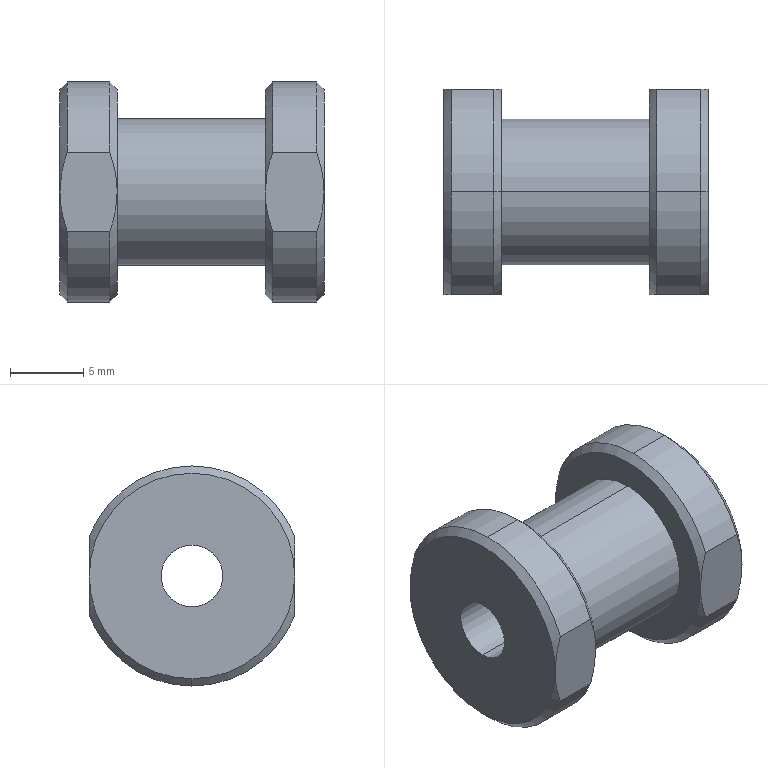Part | SolidWorks | features ICE 2, Chamfer 1, Extrusion 1, HoleWzd 1 | 1 solid | 30 faces | box 18 x 14 x 15 mm | volume 1893 mm3 | cone 12 | cylinder 10 | plane 8 | commonest cylinder face diameters 15 x6 4.2 x2 10 x2
STEP:
#1=CARTESIAN_POINT('',(3.9,0.,-5.));
#2=VERTEX_POINT('',#1);
#3=CARTESIAN_POINT('',(3.9,0.,5.));
#4=VERTEX_POINT('',#3);
#5=CARTESIAN_POINT('',(3.9,0.,0.));
#6=DIRECTION('',(1.,0.,0.));
#7=DIRECTION('',(0.,0.,-1.));
#8=AXIS2_PLACEMENT_3D('',#5,#6,#7);
#9=CIRCLE('',#8,5.);
#10=EDGE_CURVE('',#2,#4,#9,.T.);
#11=ORIENTED_EDGE('',*,*,#10,.T.);
#12=CARTESIAN_POINT('',(14.,0.,5.));
#13=VERTEX_POINT('',#12);
#14=CARTESIAN_POINT('',(3.9,0.,5.));
#15=DIRECTION('',(1.,0.,0.));
#16=VECTOR('',#15,1000.);
#17=LINE('',#14,#16);
#18=EDGE_CURVE('',#4,#13,#17,.T.);
#19=ORIENTED_EDGE('',*,*,#18,.T.);
#20=CARTESIAN_POINT('',(14.,0.,-5.));
#21=VERTEX_POINT('',#20);
#22=CARTESIAN_POINT('',(14.,0.,0.));
#23=DIRECTION('',(1.,0.,0.));
#24=DIRECTION('',(0.,0.,-1.));
#25=AXIS2_PLACEMENT_3D('',#22,#23,#24);
#26=CIRCLE('',#25,5.);
#27=EDGE_CURVE('',#21,#13,#26,.T.);
#28=ORIENTED_EDGE('',*,*,#27,.F.);
#29=CARTESIAN_POINT('',(3.9,0.,-5.));
#30=DIRECTION('',(1.,0.,0.));
#31=VECTOR('',#30,1000.);
#32=LINE('',#29,#31);
#33=EDGE_CURVE('',#2,#21,#32,.T.);
#34=ORIENTED_EDGE('',*,*,#33,.F.);
#35=EDGE_LOOP('',(#11,#19,#28,#34));
#36=FACE_OUTER_BOUND('',#35,.T.);
#37=CARTESIAN_POINT('',(3.9,0.,0.));
#38=DIRECTION('',(1.,0.,0.));
#39=DIRECTION('',(0.,0.,-1.));
#40=AXIS2_PLACEMENT_3D('',#37,#38,#39);
#41=CYLINDRICAL_SURFACE('',#40,5.);
#42=ADVANCED_FACE('',(#36),#41,.T.);
#43=CARTESIAN_POINT('',(0.,0.,2.1));
#44=VERTEX_POINT('',#43);
#45=CARTESIAN_POINT('',(0.,0.,-2.1));
#46=VERTEX_POINT('',#45);
#47=CARTESIAN_POINT('',(0.,0.,0.));
#48=DIRECTION('',(1.,0.,0.));
#49=DIRECTION('',(0.,0.,-1.));
#50=AXIS2_PLACEMENT_3D('',#47,#48,#49);
#51=CIRCLE('',#50,2.1);
#52=EDGE_CURVE('',#44,#46,#51,.T.);
#53=ORIENTED_EDGE('',*,*,#52,.F.);
#54=CARTESIAN_POINT('',(18.,0.,2.1));
#55=VERTEX_POINT('',#54);
#56=CARTESIAN_POINT('',(18.,0.,2.1));
#57=DIRECTION('',(1.,0.,0.));
#58=VECTOR('',#57,1000.);
#59=LINE('',#56,#58);
#60=EDGE_CURVE('',#44,#55,#59,.T.);
#61=ORIENTED_EDGE('',*,*,#60,.T.);
#62=CARTESIAN_POINT('',(18.,0.,-2.1));
#63=VERTEX_POINT('',#62);
#64=CARTESIAN_POINT('',(18.,0.,0.));
#65=DIRECTION('',(1.,0.,0.));
#66=DIRECTION('',(0.,0.,-1.));
#67=AXIS2_PLACEMENT_3D('',#64,#65,#66);
#68=CIRCLE('',#67,2.1);
#69=EDGE_CURVE('',#55,#63,#68,.T.);
#70=ORIENTED_EDGE('',*,*,#69,.T.);
#71=CARTESIAN_POINT('',(18.,0.,-2.1));
#72=DIRECTION('',(1.,0.,0.));
#73=VECTOR('',#72,1000.);
#74=LINE('',#71,#73);
#75=EDGE_CURVE('',#46,#63,#74,.T.);
#76=ORIENTED_EDGE('',*,*,#75,.F.);
#77=EDGE_LOOP('',(#53,#61,#70,#76));
#78=FACE_OUTER_BOUND('',#77,.T.);
#79=CARTESIAN_POINT('',(18.,0.,0.));
#80=DIRECTION('',(1.,0.,0.));
#81=DIRECTION('',(0.,0.,-1.));
#82=AXIS2_PLACEMENT_3D('',#79,#80,#81);
#83=CYLINDRICAL_SURFACE('',#82,2.1);
#84=ADVANCED_FACE('',(#78),#83,.F.);
#85=CARTESIAN_POINT('',(0.,0.,-7.));
#86=VERTEX_POINT('',#85);
#87=CARTESIAN_POINT('',(0.,-7.,0.));
#88=VERTEX_POINT('',#87);
#89=CARTESIAN_POINT('',(0.,0.,0.));
#90=DIRECTION('',(-1.,0.,0.));
#91=DIRECTION('',(0.,0.,-1.));
#92=AXIS2_PLACEMENT_3D('',#89,#90,#91);
#93=CIRCLE('',#92,7.);
#94=EDGE_CURVE('',#86,#88,#93,.T.);
#95=ORIENTED_EDGE('',*,*,#94,.F.);
#96=CARTESIAN_POINT('',(0.5,0.,-7.5));
#97=VERTEX_POINT('',#96);
#98=CARTESIAN_POINT('',(0.5,0.,-7.5));
#99=DIRECTION('',(0.7071,0.,-0.7071));
#100=VECTOR('',#99,1000.);
#101=LINE('',#98,#100);
#102=EDGE_CURVE('',#86,#97,#101,.T.);
#103=ORIENTED_EDGE('',*,*,#102,.T.);
#104=CARTESIAN_POINT('',(0.5,-7.,-2.693));
#105=VERTEX_POINT('',#104);
#106=CARTESIAN_POINT('',(0.5,0.,0.));
#107=DIRECTION('',(1.,0.,0.));
#108=DIRECTION('',(0.,0.,-1.));
#109=AXIS2_PLACEMENT_3D('',#106,#107,#108);
#110=CIRCLE('',#109,7.5);
#111=EDGE_CURVE('',#105,#97,#110,.T.);
#112=ORIENTED_EDGE('',*,*,#111,.F.);
#113=CARTESIAN_POINT('',(0.5,-7.,-2.693));
#114=CARTESIAN_POINT('',(0.3456,-7.,-2.263));
#115=CARTESIAN_POINT('',(0.2183,-7.,-1.816));
#116=CARTESIAN_POINT('',(0.04574,-7.,-0.9154));
#117=CARTESIAN_POINT('',(0.,-7.,-0.4603));
#118=CARTESIAN_POINT('',(0.,-7.,0.));
#119=B_SPLINE_CURVE_WITH_KNOTS('',3,(#113,#114,#115,#116,#117,#118),.UNSPECIFIED.,.F.,.F.,(4,2,4),(0.002778,0.004145,0.005512),.UNSPECIFIED.);
#120=EDGE_CURVE('',#105,#88,#119,.T.);
#121=ORIENTED_EDGE('',*,*,#120,.T.);
#122=EDGE_LOOP('',(#95,#103,#112,#121));
#123=FACE_OUTER_BOUND('',#122,.T.);
#124=CARTESIAN_POINT('',(0.5,0.,0.));
#125=DIRECTION('',(1.,0.,0.));
#126=DIRECTION('',(0.,0.,-1.));
#127=AXIS2_PLACEMENT_3D('',#124,#125,#126);
#128=CONICAL_SURFACE('',#127,7.5,0.7854);
#129=ADVANCED_FACE('',(#123),#128,.T.);
#130=CARTESIAN_POINT('',(3.9,0.,7.));
#131=VERTEX_POINT('',#130);
#132=CARTESIAN_POINT('',(3.9,-7.,0.));
#133=VERTEX_POINT('',#132);
#134=CARTESIAN_POINT('',(3.9,0.,0.));
#135=DIRECTION('',(1.,0.,0.));
#136=DIRECTION('',(0.,0.,-1.));
#137=AXIS2_PLACEMENT_3D('',#134,#135,#136);
#138=CIRCLE('',#137,7.);
#139=EDGE_CURVE('',#131,#133,#138,.T.);
#140=ORIENTED_EDGE('',*,*,#139,.F.);
#141=CARTESIAN_POINT('',(3.4,0.,7.5));
#142=VERTEX_POINT('',#141);
#143=CARTESIAN_POINT('',(3.9,0.,7.));
#144=DIRECTION('',(-0.7071,0.,0.7071));
#145=VECTOR('',#144,1000.);
#146=LINE('',#143,#145);
#147=EDGE_CURVE('',#131,#142,#146,.T.);
#148=ORIENTED_EDGE('',*,*,#147,.T.);
#149=CARTESIAN_POINT('',(3.4,-7.,2.693));
#150=VERTEX_POINT('',#149);
#151=CARTESIAN_POINT('',(3.4,0.,0.));
#152=DIRECTION('',(-1.,0.,0.));
#153=DIRECTION('',(0.,0.,-1.));
#154=AXIS2_PLACEMENT_3D('',#151,#152,#153);
#155=CIRCLE('',#154,7.5);
#156=EDGE_CURVE('',#150,#142,#155,.T.);
#157=ORIENTED_EDGE('',*,*,#156,.F.);
#158=CARTESIAN_POINT('',(3.4,-7.,2.693));
#159=CARTESIAN_POINT('',(3.556,-7.,2.258));
#160=CARTESIAN_POINT('',(3.681,-7.,1.818));
#161=CARTESIAN_POINT('',(3.81,-7.,1.145));
#162=CARTESIAN_POINT('',(3.844,-7.,0.919));
#163=CARTESIAN_POINT('',(3.888,-7.,0.4621));
#164=CARTESIAN_POINT('',(3.9,-7.,0.2303));
#165=CARTESIAN_POINT('',(3.9,-7.,0.));
#166=B_SPLINE_CURVE_WITH_KNOTS('',3,(#158,#159,#160,#161,#162,#163,#164,#165),.UNSPECIFIED.,.F.,.F.,(4,2,2,4),(0.006062,0.007422,0.008103,0.008783),.UNSPECIFIED.);
#167=EDGE_CURVE('',#150,#133,#166,.T.);
#168=ORIENTED_EDGE('',*,*,#167,.T.);
#169=EDGE_LOOP('',(#140,#148,#157,#168));
#170=FACE_OUTER_BOUND('',#169,.T.);
#171=CARTESIAN_POINT('',(3.9,0.,0.));
#172=DIRECTION('',(-1.,0.,0.));
#173=DIRECTION('',(0.,0.,1.));
#174=AXIS2_PLACEMENT_3D('',#171,#172,#173);
#175=CONICAL_SURFACE('',#174,7.,0.7854);
#176=ADVANCED_FACE('',(#170),#175,.T.);
#177=CARTESIAN_POINT('',(14.,0.,-7.));
#178=VERTEX_POINT('',#177);
#179=CARTESIAN_POINT('',(14.,-7.,0.));
#180=VERTEX_POINT('',#179);
#181=CARTESIAN_POINT('',(14.,0.,0.));
#182=DIRECTION('',(-1.,0.,0.));
#183=DIRECTION('',(0.,0.,-1.));
#184=AXIS2_PLACEMENT_3D('',#181,#182,#183);
#185=CIRCLE('',#184,7.);
#186=EDGE_CURVE('',#178,#180,#185,.T.);
#187=ORIENTED_EDGE('',*,*,#186,.F.);
#188=CARTESIAN_POINT('',(14.5,0.,-7.5));
#189=VERTEX_POINT('',#188);
#190=CARTESIAN_POINT('',(14.5,0.,-7.5));
#191=DIRECTION('',(0.7071,0.,-0.7071));
#192=VECTOR('',#191,1000.);
#193=LINE('',#190,#192);
#194=EDGE_CURVE('',#178,#189,#193,.T.);
#195=ORIENTED_EDGE('',*,*,#194,.T.);
#196=CARTESIAN_POINT('',(14.5,-7.,-2.693));
#197=VERTEX_POINT('',#196);
#198=CARTESIAN_POINT('',(14.5,0.,0.));
#199=DIRECTION('',(1.,0.,0.));
#200=DIRECTION('',(0.,0.,-1.));
#201=AXIS2_PLACEMENT_3D('',#198,#199,#200);
#202=CIRCLE('',#201,7.5);
#203=EDGE_CURVE('',#197,#189,#202,.T.);
#204=ORIENTED_EDGE('',*,*,#203,.F.);
#205=CARTESIAN_POINT('',(14.5,-7.,-2.693));
#206=CARTESIAN_POINT('',(14.346,-7.,-2.263));
#207=CARTESIAN_POINT('',(14.218,-7.,-1.816));
#208=CARTESIAN_POINT('',(14.046,-7.,-0.9154));
#209=CARTESIAN_POINT('',(14.,-7.,-0.4603));
#210=CARTESIAN_POINT('',(14.,-7.,0.));
#211=B_SPLINE_CURVE_WITH_KNOTS('',3,(#205,#206,#207,#208,#209,#210),.UNSPECIFIED.,.F.,.F.,(4,2,4),(0.002778,0.004145,0.005512),.UNSPECIFIED.);
#212=EDGE_CURVE('',#197,#180,#211,.T.);
#213=ORIENTED_EDGE('',*,*,#212,.T.);
#214=EDGE_LOOP('',(#187,#195,#204,#213));
#215=FACE_OUTER_BOUND('',#214,.T.);
#216=CARTESIAN_POINT('',(14.5,0.,0.));
#217=DIRECTION('',(1.,0.,0.));
#218=DIRECTION('',(0.,0.,-1.));
#219=AXIS2_PLACEMENT_3D('',#216,#217,#218);
#220=CONICAL_SURFACE('',#219,7.5,0.7854);
#221=ADVANCED_FACE('',(#215),#220,.T.);
#222=CARTESIAN_POINT('',(18.,0.,7.));
#223=VERTEX_POINT('',#222);
#224=CARTESIAN_POINT('',(18.,-7.,0.));
#225=VERTEX_POINT('',#224);
#226=CARTESIAN_POINT('',(18.,0.,0.));
#227=DIRECTION('',(1.,0.,0.));
#228=DIRECTION('',(0.,0.,-1.));
#229=AXIS2_PLACEMENT_3D('',#226,#227,#228);
#230=CIRCLE('',#229,7.);
#231=EDGE_CURVE('',#223,#225,#230,.T.);
#232=ORIENTED_EDGE('',*,*,#231,.F.);
#233=CARTESIAN_POINT('',(17.5,0.,7.5));
#234=VERTEX_POINT('',#233);
#235=CARTESIAN_POINT('',(18.,0.,7.));
#236=DIRECTION('',(-0.7071,0.,0.7071));
#237=VECTOR('',#236,1000.);
#238=LINE('',#235,#237);
#239=EDGE_CURVE('',#223,#234,#238,.T.);
#240=ORIENTED_EDGE('',*,*,#239,.T.);
#241=CARTESIAN_POINT('',(17.5,-7.,2.693));
#242=VERTEX_POINT('',#241);
#243=CARTESIAN_POINT('',(17.5,0.,0.));
#244=DIRECTION('',(-1.,0.,0.));
#245=DIRECTION('',(0.,0.,-1.));
#246=AXIS2_PLACEMENT_3D('',#243,#244,#245);
#247=CIRCLE('',#246,7.5);
#248=EDGE_CURVE('',#242,#234,#247,.T.);
#249=ORIENTED_EDGE('',*,*,#248,.F.);
#250=CARTESIAN_POINT('',(17.5,-7.,2.693));
#251=CARTESIAN_POINT('',(17.656,-7.,2.258));
#252=CARTESIAN_POINT('',(17.781,-7.,1.818));
#253=CARTESIAN_POINT('',(17.91,-7.,1.145));
#254=CARTESIAN_POINT('',(17.944,-7.,0.919));
#255=CARTESIAN_POINT('',(17.988,-7.,0.4621));
#256=CARTESIAN_POINT('',(18.,-7.,0.2303));
#257=CARTESIAN_POINT('',(18.,-7.,0.));
#258=B_SPLINE_CURVE_WITH_KNOTS('',3,(#250,#251,#252,#253,#254,#255,#256,#257),.UNSPECIFIED.,.F.,.F.,(4,2,2,4),(0.006062,0.007422,0.008103,0.008783),.UNSPECIFIED.);
#259=EDGE_CURVE('',#242,#225,#258,.T.);
#260=ORIENTED_EDGE('',*,*,#259,.T.);
#261=EDGE_LOOP('',(#232,#240,#249,#260));
#262=FACE_OUTER_BOUND('',#261,.T.);
#263=CARTESIAN_POINT('',(18.,0.,0.));
#264=DIRECTION('',(-1.,0.,0.));
#265=DIRECTION('',(0.,0.,1.));
#266=AXIS2_PLACEMENT_3D('',#263,#264,#265);
#267=CONICAL_SURFACE('',#266,7.,0.7854);
#268=ADVANCED_FACE('',(#262),#267,.T.);
#269=ORIENTED_EDGE('',*,*,#248,.T.);
#270=CARTESIAN_POINT('',(14.5,0.,7.5));
#271=VERTEX_POINT('',#270);
#272=CARTESIAN_POINT('',(18.,0.,7.5));
#273=DIRECTION('',(-1.,0.,0.));
#274=VECTOR('',#273,1000.);
#275=LINE('',#272,#274);
#276=EDGE_CURVE('',#234,#271,#275,.T.);
#277=ORIENTED_EDGE('',*,*,#276,.T.);
#278=CARTESIAN_POINT('',(14.5,-7.,2.693));
#279=VERTEX_POINT('',#278);
#280=CARTESIAN_POINT('',(14.5,0.,0.));
#281=DIRECTION('',(1.,0.,0.));
#282=DIRECTION('',(0.,0.,-1.));
#283=AXIS2_PLACEMENT_3D('',#280,#281,#282);
#284=CIRCLE('',#283,7.5);
#285=EDGE_CURVE('',#271,#279,#284,.T.);
#286=ORIENTED_EDGE('',*,*,#285,.T.);
#287=CARTESIAN_POINT('',(18.,-7.,2.693));
#288=DIRECTION('',(-1.,0.,0.));
#289=VECTOR('',#288,1000.);
#290=LINE('',#287,#289);
#291=EDGE_CURVE('',#242,#279,#290,.T.);
#292=ORIENTED_EDGE('',*,*,#291,.F.);
#293=EDGE_LOOP('',(#269,#277,#286,#292));
#294=FACE_OUTER_BOUND('',#293,.T.);
#295=CARTESIAN_POINT('',(18.,0.,0.));
#296=DIRECTION('',(-1.,0.,0.));
#297=DIRECTION('',(0.,0.,1.));
#298=AXIS2_PLACEMENT_3D('',#295,#296,#297);
#299=CYLINDRICAL_SURFACE('',#298,7.5);
#300=ADVANCED_FACE('',(#294),#299,.T.);
#301=ORIENTED_EDGE('',*,*,#156,.T.);
#302=CARTESIAN_POINT('',(0.5,0.,7.5));
#303=VERTEX_POINT('',#302);
#304=CARTESIAN_POINT('',(18.,0.,7.5));
#305=DIRECTION('',(-1.,0.,0.));
#306=VECTOR('',#305,1000.);
#307=LINE('',#304,#306);
#308=EDGE_CURVE('',#142,#303,#307,.T.);
#309=ORIENTED_EDGE('',*,*,#308,.T.);
#310=CARTESIAN_POINT('',(0.5,-7.,2.693));
#311=VERTEX_POINT('',#310);
#312=CARTESIAN_POINT('',(0.5,0.,0.));
#313=DIRECTION('',(1.,0.,0.));
#314=DIRECTION('',(0.,0.,-1.));
#315=AXIS2_PLACEMENT_3D('',#312,#313,#314);
#316=CIRCLE('',#315,7.5);
#317=EDGE_CURVE('',#303,#311,#316,.T.);
#318=ORIENTED_EDGE('',*,*,#317,.T.);
#319=CARTESIAN_POINT('',(18.,-7.,2.693));
#320=DIRECTION('',(-1.,0.,0.));
#321=VECTOR('',#320,1000.);
#322=LINE('',#319,#321);
#323=EDGE_CURVE('',#150,#311,#322,.T.);
#324=ORIENTED_EDGE('',*,*,#323,.F.);
#325=EDGE_LOOP('',(#301,#309,#318,#324));
#326=FACE_OUTER_BOUND('',#325,.T.);
#327=CARTESIAN_POINT('',(18.,0.,0.));
#328=DIRECTION('',(-1.,0.,0.));
#329=DIRECTION('',(0.,0.,1.));
#330=AXIS2_PLACEMENT_3D('',#327,#328,#329);
#331=CYLINDRICAL_SURFACE('',#330,7.5);
#332=ADVANCED_FACE('',(#326),#331,.T.);
#333=ORIENTED_EDGE('',*,*,#308,.F.);
#334=CARTESIAN_POINT('',(3.4,7.,2.693));
#335=VERTEX_POINT('',#334);
#336=CARTESIAN_POINT('',(3.4,0.,0.));
#337=DIRECTION('',(-1.,0.,0.));
#338=DIRECTION('',(0.,0.,-1.));
#339=AXIS2_PLACEMENT_3D('',#336,#337,#338);
#340=CIRCLE('',#339,7.5);
#341=EDGE_CURVE('',#142,#335,#340,.T.);
#342=ORIENTED_EDGE('',*,*,#341,.T.);
#343=CARTESIAN_POINT('',(0.5,7.,2.693));
#344=VERTEX_POINT('',#343);
#345=CARTESIAN_POINT('',(18.,7.,2.693));
#346=DIRECTION('',(1.,0.,0.));
#347=VECTOR('',#346,1000.);
#348=LINE('',#345,#347);
#349=EDGE_CURVE('',#344,#335,#348,.T.);
#350=ORIENTED_EDGE('',*,*,#349,.F.);
#351=CARTESIAN_POINT('',(0.5,0.,0.));
#352=DIRECTION('',(1.,0.,0.));
#353=DIRECTION('',(0.,0.,-1.));
#354=AXIS2_PLACEMENT_3D('',#351,#352,#353);
#355=CIRCLE('',#354,7.5);
#356=EDGE_CURVE('',#344,#303,#355,.T.);
#357=ORIENTED_EDGE('',*,*,#356,.T.);
#358=EDGE_LOOP('',(#333,#342,#350,#357));
#359=FACE_OUTER_BOUND('',#358,.T.);
#360=CARTESIAN_POINT('',(18.,0.,0.));
#361=DIRECTION('',(-1.,0.,0.));
#362=DIRECTION('',(0.,0.,1.));
#363=AXIS2_PLACEMENT_3D('',#360,#361,#362);
#364=CYLINDRICAL_SURFACE('',#363,7.5);
#365=ADVANCED_FACE('',(#359),#364,.T.);
#366=CARTESIAN_POINT('',(3.4,-7.,-2.693));
#367=VERTEX_POINT('',#366);
#368=CARTESIAN_POINT('',(18.,-7.,-2.693));
#369=DIRECTION('',(1.,0.,0.));
#370=VECTOR('',#369,1000.);
#371=LINE('',#368,#370);
#372=EDGE_CURVE('',#105,#367,#371,.T.);
#373=ORIENTED_EDGE('',*,*,#372,.F.);
#374=ORIENTED_EDGE('',*,*,#111,.T.);
#375=CARTESIAN_POINT('',(0.5,7.,-2.693));
#376=VERTEX_POINT('',#375);
#377=CARTESIAN_POINT('',(0.5,0.,0.));
#378=DIRECTION('',(1.,0.,0.));
#379=DIRECTION('',(0.,0.,-1.));
#380=AXIS2_PLACEMENT_3D('',#377,#378,#379);
#381=CIRCLE('',#380,7.5);
#382=EDGE_CURVE('',#97,#376,#381,.T.);
#383=ORIENTED_EDGE('',*,*,#382,.T.);
#384=CARTESIAN_POINT('',(3.4,7.,-2.693));
#385=VERTEX_POINT('',#384);
#386=CARTESIAN_POINT('',(18.,7.,-2.693));
#387=DIRECTION('',(-1.,0.,0.));
#388=VECTOR('',#387,1000.);
#389=LINE('',#386,#388);
#390=EDGE_CURVE('',#385,#376,#389,.T.);
#391=ORIENTED_EDGE('',*,*,#390,.F.);
#392=CARTESIAN_POINT('',(3.4,0.,0.));
#393=DIRECTION('',(-1.,0.,0.));
#394=DIRECTION('',(0.,0.,-1.));
#395=AXIS2_PLACEMENT_3D('',#392,#393,#394);
#396=CIRCLE('',#395,7.5);
#397=EDGE_CURVE('',#385,#367,#396,.T.);
#398=ORIENTED_EDGE('',*,*,#397,.T.);
#399=EDGE_LOOP('',(#373,#374,#383,#391,#398));
#400=FACE_OUTER_BOUND('',#399,.T.);
#401=CARTESIAN_POINT('',(18.,0.,0.));
#402=DIRECTION('',(-1.,0.,0.));
#403=DIRECTION('',(0.,0.,1.));
#404=AXIS2_PLACEMENT_3D('',#401,#402,#403);
#405=CYLINDRICAL_SURFACE('',#404,7.5);
#406=ADVANCED_FACE('',(#400),#405,.T.);
#407=ORIENTED_EDGE('',*,*,#276,.F.);
#408=CARTESIAN_POINT('',(17.5,7.,2.693));
#409=VERTEX_POINT('',#408);
#410=CARTESIAN_POINT('',(17.5,0.,0.));
#411=DIRECTION('',(-1.,0.,0.));
#412=DIRECTION('',(0.,0.,-1.));
#413=AXIS2_PLACEMENT_3D('',#410,#411,#412);
#414=CIRCLE('',#413,7.5);
#415=EDGE_CURVE('',#234,#409,#414,.T.);
#416=ORIENTED_EDGE('',*,*,#415,.T.);
#417=CARTESIAN_POINT('',(14.5,7.,2.693));
#418=VERTEX_POINT('',#417);
#419=CARTESIAN_POINT('',(18.,7.,2.693));
#420=DIRECTION('',(1.,0.,0.));
#421=VECTOR('',#420,1000.);
#422=LINE('',#419,#421);
#423=EDGE_CURVE('',#418,#409,#422,.T.);
#424=ORIENTED_EDGE('',*,*,#423,.F.);
#425=CARTESIAN_POINT('',(14.5,0.,0.));
#426=DIRECTION('',(1.,0.,0.));
#427=DIRECTION('',(0.,0.,-1.));
#428=AXIS2_PLACEMENT_3D('',#425,#426,#427);
#429=CIRCLE('',#428,7.5);
#430=EDGE_CURVE('',#418,#271,#429,.T.);
#431=ORIENTED_EDGE('',*,*,#430,.T.);
#432=EDGE_LOOP('',(#407,#416,#424,#431));
#433=FACE_OUTER_BOUND('',#432,.T.);
#434=CARTESIAN_POINT('',(18.,0.,0.));
#435=DIRECTION('',(-1.,0.,0.));
#436=DIRECTION('',(0.,0.,1.));
#437=AXIS2_PLACEMENT_3D('',#434,#435,#436);
#438=CYLINDRICAL_SURFACE('',#437,7.5);
#439=ADVANCED_FACE('',(#433),#438,.T.);
#440=CARTESIAN_POINT('',(17.5,-7.,-2.693));
#441=VERTEX_POINT('',#440);
#442=CARTESIAN_POINT('',(18.,-7.,-2.693));
#443=DIRECTION('',(1.,0.,0.));
#444=VECTOR('',#443,1000.);
#445=LINE('',#442,#444);
#446=EDGE_CURVE('',#197,#441,#445,.T.);
#447=ORIENTED_EDGE('',*,*,#446,.F.);
#448=ORIENTED_EDGE('',*,*,#203,.T.);
#449=CARTESIAN_POINT('',(14.5,7.,-2.693));
#450=VERTEX_POINT('',#449);
#451=CARTESIAN_POINT('',(14.5,0.,0.));
#452=DIRECTION('',(1.,0.,0.));
#453=DIRECTION('',(0.,0.,-1.));
#454=AXIS2_PLACEMENT_3D('',#451,#452,#453);
#455=CIRCLE('',#454,7.5);
#456=EDGE_CURVE('',#189,#450,#455,.T.);
#457=ORIENTED_EDGE('',*,*,#456,.T.);
#458=CARTESIAN_POINT('',(17.5,7.,-2.693));
#459=VERTEX_POINT('',#458);
#460=CARTESIAN_POINT('',(18.,7.,-2.693));
#461=DIRECTION('',(-1.,0.,0.));
#462=VECTOR('',#461,1000.);
#463=LINE('',#460,#462);
#464=EDGE_CURVE('',#459,#450,#463,.T.);
#465=ORIENTED_EDGE('',*,*,#464,.F.);
#466=CARTESIAN_POINT('',(17.5,0.,0.));
#467=DIRECTION('',(-1.,0.,0.));
#468=DIRECTION('',(0.,0.,-1.));
#469=AXIS2_PLACEMENT_3D('',#466,#467,#468);
#470=CIRCLE('',#469,7.5);
#471=EDGE_CURVE('',#459,#441,#470,.T.);
#472=ORIENTED_EDGE('',*,*,#471,.T.);
#473=EDGE_LOOP('',(#447,#448,#457,#465,#472));
#474=FACE_OUTER_BOUND('',#473,.T.);
#475=CARTESIAN_POINT('',(18.,0.,0.));
#476=DIRECTION('',(-1.,0.,0.));
#477=DIRECTION('',(0.,0.,1.));
#478=AXIS2_PLACEMENT_3D('',#475,#476,#477);
#479=CYLINDRICAL_SURFACE('',#478,7.5);
#480=ADVANCED_FACE('',(#474),#479,.T.);
#481=ORIENTED_EDGE('',*,*,#239,.F.);
#482=CARTESIAN_POINT('',(18.,7.,0.));
#483=VERTEX_POINT('',#482);
#484=CARTESIAN_POINT('',(18.,0.,0.));
#485=DIRECTION('',(1.,0.,0.));
#486=DIRECTION('',(0.,0.,-1.));
#487=AXIS2_PLACEMENT_3D('',#484,#485,#486);
#488=CIRCLE('',#487,7.);
#489=EDGE_CURVE('',#483,#223,#488,.T.);
#490=ORIENTED_EDGE('',*,*,#489,.F.);
#491=CARTESIAN_POINT('',(18.,7.,0.));
#492=CARTESIAN_POINT('',(18.,7.,0.2303));
#493=CARTESIAN_POINT('',(17.988,7.,0.4621));
#494=CARTESIAN_POINT('',(17.944,7.,0.919));
#495=CARTESIAN_POINT('',(17.91,7.,1.145));
#496=CARTESIAN_POINT('',(17.781,7.,1.818));
#497=CARTESIAN_POINT('',(17.656,7.,2.258));
#498=CARTESIAN_POINT('',(17.5,7.,2.693));
#499=B_SPLINE_CURVE_WITH_KNOTS('',3,(#491,#492,#493,#494,#495,#496,#497,#498),.UNSPECIFIED.,.F.,.F.,(4,2,2,4),(0.005512,0.006196,0.00688,0.008248),.UNSPECIFIED.);
#500=EDGE_CURVE('',#483,#409,#499,.T.);
#501=ORIENTED_EDGE('',*,*,#500,.T.);
#502=ORIENTED_EDGE('',*,*,#415,.F.);
#503=EDGE_LOOP('',(#481,#490,#501,#502));
#504=FACE_OUTER_BOUND('',#503,.T.);
#505=CARTESIAN_POINT('',(18.,0.,0.));
#506=DIRECTION('',(-1.,0.,0.));
#507=DIRECTION('',(0.,0.,1.));
#508=AXIS2_PLACEMENT_3D('',#505,#506,#507);
#509=CONICAL_SURFACE('',#508,7.,0.7854);
#510=ADVANCED_FACE('',(#504),#509,.T.);
#511=CARTESIAN_POINT('',(18.,0.,0.));
#512=DIRECTION('',(1.,0.,0.));
#513=DIRECTION('',(0.,0.,-1.));
#514=AXIS2_PLACEMENT_3D('',#511,#512,#513);
#515=CIRCLE('',#514,7.);
#516=EDGE_CURVE('',#225,#483,#515,.T.);
#517=ORIENTED_EDGE('',*,*,#516,.F.);
#518=CARTESIAN_POINT('',(18.,-7.,0.));
#519=CARTESIAN_POINT('',(18.,-7.,-0.4603));
#520=CARTESIAN_POINT('',(17.954,-7.,-0.9154));
#521=CARTESIAN_POINT('',(17.782,-7.,-1.816));
#522=CARTESIAN_POINT('',(17.654,-7.,-2.263));
#523=CARTESIAN_POINT('',(17.5,-7.,-2.693));
#524=B_SPLINE_CURVE_WITH_KNOTS('',3,(#518,#519,#520,#521,#522,#523),.UNSPECIFIED.,.F.,.F.,(4,2,4),(0.008783,0.01014,0.0115),.UNSPECIFIED.);
#525=EDGE_CURVE('',#225,#441,#524,.T.);
#526=ORIENTED_EDGE('',*,*,#525,.T.);
#527=ORIENTED_EDGE('',*,*,#471,.F.);
#528=CARTESIAN_POINT('',(17.5,7.,-2.693));
#529=CARTESIAN_POINT('',(17.654,7.,-2.263));
#530=CARTESIAN_POINT('',(17.782,7.,-1.816));
#531=CARTESIAN_POINT('',(17.954,7.,-0.9154));
#532=CARTESIAN_POINT('',(18.,7.,-0.4603));
#533=CARTESIAN_POINT('',(18.,7.,0.));
#534=B_SPLINE_CURVE_WITH_KNOTS('',3,(#528,#529,#530,#531,#532,#533),.UNSPECIFIED.,.F.,.F.,(4,2,4),(0.002778,0.004145,0.005512),.UNSPECIFIED.);
#535=EDGE_CURVE('',#459,#483,#534,.T.);
#536=ORIENTED_EDGE('',*,*,#535,.T.);
#537=EDGE_LOOP('',(#517,#526,#527,#536));
#538=FACE_OUTER_BOUND('',#537,.T.);
#539=CARTESIAN_POINT('',(18.,0.,0.));
#540=DIRECTION('',(-1.,0.,0.));
#541=DIRECTION('',(0.,0.,1.));
#542=AXIS2_PLACEMENT_3D('',#539,#540,#541);
#543=CONICAL_SURFACE('',#542,7.,0.7854);
#544=ADVANCED_FACE('',(#538),#543,.T.);
#545=ORIENTED_EDGE('',*,*,#194,.F.);
#546=CARTESIAN_POINT('',(14.,7.,0.));
#547=VERTEX_POINT('',#546);
#548=CARTESIAN_POINT('',(14.,0.,0.));
#549=DIRECTION('',(-1.,0.,0.));
#550=DIRECTION('',(0.,0.,-1.));
#551=AXIS2_PLACEMENT_3D('',#548,#549,#550);
#552=CIRCLE('',#551,7.);
#553=EDGE_CURVE('',#547,#178,#552,.T.);
#554=ORIENTED_EDGE('',*,*,#553,.F.);
#555=CARTESIAN_POINT('',(14.,7.,0.));
#556=CARTESIAN_POINT('',(14.,7.,-0.4603));
#557=CARTESIAN_POINT('',(14.046,7.,-0.9154));
#558=CARTESIAN_POINT('',(14.218,7.,-1.816));
#559=CARTESIAN_POINT('',(14.346,7.,-2.263));
#560=CARTESIAN_POINT('',(14.5,7.,-2.693));
#561=B_SPLINE_CURVE_WITH_KNOTS('',3,(#555,#556,#557,#558,#559,#560),.UNSPECIFIED.,.F.,.F.,(4,2,4),(0.008783,0.01014,0.0115),.UNSPECIFIED.);
#562=EDGE_CURVE('',#547,#450,#561,.T.);
#563=ORIENTED_EDGE('',*,*,#562,.T.);
#564=ORIENTED_EDGE('',*,*,#456,.F.);
#565=EDGE_LOOP('',(#545,#554,#563,#564));
#566=FACE_OUTER_BOUND('',#565,.T.);
#567=CARTESIAN_POINT('',(14.5,0.,0.));
#568=DIRECTION('',(1.,0.,0.));
#569=DIRECTION('',(0.,0.,-1.));
#570=AXIS2_PLACEMENT_3D('',#567,#568,#569);
#571=CONICAL_SURFACE('',#570,7.5,0.7854);
#572=ADVANCED_FACE('',(#566),#571,.T.);
#573=CARTESIAN_POINT('',(14.,0.,0.));
#574=DIRECTION('',(-1.,0.,0.));
#575=DIRECTION('',(0.,0.,-1.));
#576=AXIS2_PLACEMENT_3D('',#573,#574,#575);
#577=CIRCLE('',#576,7.);
#578=EDGE_CURVE('',#180,#547,#577,.T.);
#579=ORIENTED_EDGE('',*,*,#578,.F.);
#580=CARTESIAN_POINT('',(14.,-7.,0.));
#581=CARTESIAN_POINT('',(14.,-7.,0.2303));
#582=CARTESIAN_POINT('',(14.012,-7.,0.4621));
#583=CARTESIAN_POINT('',(14.056,-7.,0.919));
#584=CARTESIAN_POINT('',(14.09,-7.,1.145));
#585=CARTESIAN_POINT('',(14.219,-7.,1.818));
#586=CARTESIAN_POINT('',(14.344,-7.,2.258));
#587=CARTESIAN_POINT('',(14.5,-7.,2.693));
#588=B_SPLINE_CURVE_WITH_KNOTS('',3,(#580,#581,#582,#583,#584,#585,#586,#587),.UNSPECIFIED.,.F.,.F.,(4,2,2,4),(0.005512,0.006196,0.00688,0.008248),.UNSPECIFIED.);
#589=EDGE_CURVE('',#180,#279,#588,.T.);
#590=ORIENTED_EDGE('',*,*,#589,.T.);
#591=ORIENTED_EDGE('',*,*,#285,.F.);
#592=ORIENTED_EDGE('',*,*,#430,.F.);
#593=CARTESIAN_POINT('',(14.5,7.,2.693));
#594=CARTESIAN_POINT('',(14.344,7.,2.258));
#595=CARTESIAN_POINT('',(14.219,7.,1.818));
#596=CARTESIAN_POINT('',(14.09,7.,1.145));
#597=CARTESIAN_POINT('',(14.056,7.,0.919));
#598=CARTESIAN_POINT('',(14.012,7.,0.4621));
#599=CARTESIAN_POINT('',(14.,7.,0.2303));
#600=CARTESIAN_POINT('',(14.,7.,0.));
#601=B_SPLINE_CURVE_WITH_KNOTS('',3,(#593,#594,#595,#596,#597,#598,#599,#600),.UNSPECIFIED.,.F.,.F.,(4,2,2,4),(0.006062,0.007422,0.008103,0.008783),.UNSPECIFIED.);
#602=EDGE_CURVE('',#418,#547,#601,.T.);
#603=ORIENTED_EDGE('',*,*,#602,.T.);
#604=EDGE_LOOP('',(#579,#590,#591,#592,#603));
#605=FACE_OUTER_BOUND('',#604,.T.);
#606=CARTESIAN_POINT('',(14.5,0.,0.));
#607=DIRECTION('',(1.,0.,0.));
#608=DIRECTION('',(0.,0.,-1.));
#609=AXIS2_PLACEMENT_3D('',#606,#607,#608);
#610=CONICAL_SURFACE('',#609,7.5,0.7854);
#611=ADVANCED_FACE('',(#605),#610,.T.);
#612=ORIENTED_EDGE('',*,*,#147,.F.);
#613=CARTESIAN_POINT('',(3.9,7.,0.));
#614=VERTEX_POINT('',#613);
#615=CARTESIAN_POINT('',(3.9,0.,0.));
#616=DIRECTION('',(1.,0.,0.));
#617=DIRECTION('',(0.,0.,-1.));
#618=AXIS2_PLACEMENT_3D('',#615,#616,#617);
#619=CIRCLE('',#618,7.);
#620=EDGE_CURVE('',#614,#131,#619,.T.);
#621=ORIENTED_EDGE('',*,*,#620,.F.);
#622=CARTESIAN_POINT('',(3.9,7.,0.));
#623=CARTESIAN_POINT('',(3.9,7.,0.2303));
#624=CARTESIAN_POINT('',(3.888,7.,0.4621));
#625=CARTESIAN_POINT('',(3.844,7.,0.919));
#626=CARTESIAN_POINT('',(3.81,7.,1.145));
#627=CARTESIAN_POINT('',(3.681,7.,1.818));
#628=CARTESIAN_POINT('',(3.556,7.,2.258));
#629=CARTESIAN_POINT('',(3.4,7.,2.693));
#630=B_SPLINE_CURVE_WITH_KNOTS('',3,(#622,#623,#624,#625,#626,#627,#628,#629),.UNSPECIFIED.,.F.,.F.,(4,2,2,4),(0.005512,0.006196,0.00688,0.008248),.UNSPECIFIED.);
#631=EDGE_CURVE('',#614,#335,#630,.T.);
#632=ORIENTED_EDGE('',*,*,#631,.T.);
#633=ORIENTED_EDGE('',*,*,#341,.F.);
#634=EDGE_LOOP('',(#612,#621,#632,#633));
#635=FACE_OUTER_BOUND('',#634,.T.);
#636=CARTESIAN_POINT('',(3.9,0.,0.));
#637=DIRECTION('',(-1.,0.,0.));
#638=DIRECTION('',(0.,0.,1.));
#639=AXIS2_PLACEMENT_3D('',#636,#637,#638);
#640=CONICAL_SURFACE('',#639,7.,0.7854);
#641=ADVANCED_FACE('',(#635),#640,.T.);
#642=CARTESIAN_POINT('',(3.9,0.,0.));
#643=DIRECTION('',(1.,0.,0.));
#644=DIRECTION('',(0.,0.,-1.));
#645=AXIS2_PLACEMENT_3D('',#642,#643,#644);
#646=CIRCLE('',#645,7.);
#647=EDGE_CURVE('',#133,#614,#646,.T.);
#648=ORIENTED_EDGE('',*,*,#647,.F.);
#649=CARTESIAN_POINT('',(3.9,-7.,0.));
#650=CARTESIAN_POINT('',(3.9,-7.,-0.4603));
#651=CARTESIAN_POINT('',(3.854,-7.,-0.9154));
#652=CARTESIAN_POINT('',(3.682,-7.,-1.816));
#653=CARTESIAN_POINT('',(3.554,-7.,-2.263));
#654=CARTESIAN_POINT('',(3.4,-7.,-2.693));
#655=B_SPLINE_CURVE_WITH_KNOTS('',3,(#649,#650,#651,#652,#653,#654),.UNSPECIFIED.,.F.,.F.,(4,2,4),(0.008783,0.01014,0.0115),.UNSPECIFIED.);
#656=EDGE_CURVE('',#133,#367,#655,.T.);
#657=ORIENTED_EDGE('',*,*,#656,.T.);
#658=ORIENTED_EDGE('',*,*,#397,.F.);
#659=CARTESIAN_POINT('',(3.4,7.,-2.693));
#660=CARTESIAN_POINT('',(3.554,7.,-2.263));
#661=CARTESIAN_POINT('',(3.682,7.,-1.816));
#662=CARTESIAN_POINT('',(3.854,7.,-0.9154));
#663=CARTESIAN_POINT('',(3.9,7.,-0.4603));
#664=CARTESIAN_POINT('',(3.9,7.,0.));
#665=B_SPLINE_CURVE_WITH_KNOTS('',3,(#659,#660,#661,#662,#663,#664),.UNSPECIFIED.,.F.,.F.,(4,2,4),(0.002778,0.004145,0.005512),.UNSPECIFIED.);
#666=EDGE_CURVE('',#385,#614,#665,.T.);
#667=ORIENTED_EDGE('',*,*,#666,.T.);
#668=EDGE_LOOP('',(#648,#657,#658,#667));
#669=FACE_OUTER_BOUND('',#668,.T.);
#670=CARTESIAN_POINT('',(3.9,0.,0.));
#671=DIRECTION('',(-1.,0.,0.));
#672=DIRECTION('',(0.,0.,1.));
#673=AXIS2_PLACEMENT_3D('',#670,#671,#672);
#674=CONICAL_SURFACE('',#673,7.,0.7854);
#675=ADVANCED_FACE('',(#669),#674,.T.);
#676=ORIENTED_EDGE('',*,*,#102,.F.);
#677=CARTESIAN_POINT('',(0.,7.,0.));
#678=VERTEX_POINT('',#677);
#679=CARTESIAN_POINT('',(0.,0.,0.));
#680=DIRECTION('',(-1.,0.,0.));
#681=DIRECTION('',(0.,0.,-1.));
#682=AXIS2_PLACEMENT_3D('',#679,#680,#681);
#683=CIRCLE('',#682,7.);
#684=EDGE_CURVE('',#678,#86,#683,.T.);
#685=ORIENTED_EDGE('',*,*,#684,.F.);
#686=CARTESIAN_POINT('',(0.,7.,0.));
#687=CARTESIAN_POINT('',(0.,7.,-0.4603));
#688=CARTESIAN_POINT('',(0.04574,7.,-0.9154));
#689=CARTESIAN_POINT('',(0.2183,7.,-1.816));
#690=CARTESIAN_POINT('',(0.3456,7.,-2.263));
#691=CARTESIAN_POINT('',(0.5,7.,-2.693));
#692=B_SPLINE_CURVE_WITH_KNOTS('',3,(#686,#687,#688,#689,#690,#691),.UNSPECIFIED.,.F.,.F.,(4,2,4),(0.008783,0.01014,0.0115),.UNSPECIFIED.);
#693=EDGE_CURVE('',#678,#376,#692,.T.);
#694=ORIENTED_EDGE('',*,*,#693,.T.);
#695=ORIENTED_EDGE('',*,*,#382,.F.);
#696=EDGE_LOOP('',(#676,#685,#694,#695));
#697=FACE_OUTER_BOUND('',#696,.T.);
#698=CARTESIAN_POINT('',(0.5,0.,0.));
#699=DIRECTION('',(1.,0.,0.));
#700=DIRECTION('',(0.,0.,-1.));
#701=AXIS2_PLACEMENT_3D('',#698,#699,#700);
#702=CONICAL_SURFACE('',#701,7.5,0.7854);
#703=ADVANCED_FACE('',(#697),#702,.T.);
#704=CARTESIAN_POINT('',(0.,0.,0.));
#705=DIRECTION('',(-1.,0.,0.));
#706=DIRECTION('',(0.,0.,-1.));
#707=AXIS2_PLACEMENT_3D('',#704,#705,#706);
#708=CIRCLE('',#707,7.);
#709=EDGE_CURVE('',#88,#678,#708,.T.);
#710=ORIENTED_EDGE('',*,*,#709,.F.);
#711=CARTESIAN_POINT('',(0.,-7.,0.));
#712=CARTESIAN_POINT('',(0.,-7.,0.2303));
#713=CARTESIAN_POINT('',(0.01156,-7.,0.4621));
#714=CARTESIAN_POINT('',(0.05641,-7.,0.919));
#715=CARTESIAN_POINT('',(0.08965,-7.,1.145));
#716=CARTESIAN_POINT('',(0.2188,-7.,1.818));
#717=CARTESIAN_POINT('',(0.3441,-7.,2.258));
#718=CARTESIAN_POINT('',(0.5,-7.,2.693));
#719=B_SPLINE_CURVE_WITH_KNOTS('',3,(#711,#712,#713,#714,#715,#716,#717,#718),.UNSPECIFIED.,.F.,.F.,(4,2,2,4),(0.005512,0.006196,0.00688,0.008248),.UNSPECIFIED.);
#720=EDGE_CURVE('',#88,#311,#719,.T.);
#721=ORIENTED_EDGE('',*,*,#720,.T.);
#722=ORIENTED_EDGE('',*,*,#317,.F.);
#723=ORIENTED_EDGE('',*,*,#356,.F.);
#724=CARTESIAN_POINT('',(0.5,7.,2.693));
#725=CARTESIAN_POINT('',(0.3441,7.,2.258));
#726=CARTESIAN_POINT('',(0.2188,7.,1.818));
#727=CARTESIAN_POINT('',(0.08965,7.,1.145));
#728=CARTESIAN_POINT('',(0.05641,7.,0.919));
#729=CARTESIAN_POINT('',(0.01156,7.,0.4621));
#730=CARTESIAN_POINT('',(0.,7.,0.2303));
#731=CARTESIAN_POINT('',(0.,7.,0.));
#732=B_SPLINE_CURVE_WITH_KNOTS('',3,(#724,#725,#726,#727,#728,#729,#730,#731),.UNSPECIFIED.,.F.,.F.,(4,2,2,4),(0.006062,0.007422,0.008103,0.008783),.UNSPECIFIED.);
#733=EDGE_CURVE('',#344,#678,#732,.T.);
#734=ORIENTED_EDGE('',*,*,#733,.T.);
#735=EDGE_LOOP('',(#710,#721,#722,#723,#734));
#736=FACE_OUTER_BOUND('',#735,.T.);
#737=CARTESIAN_POINT('',(0.5,0.,0.));
#738=DIRECTION('',(1.,0.,0.));
#739=DIRECTION('',(0.,0.,-1.));
#740=AXIS2_PLACEMENT_3D('',#737,#738,#739);
#741=CONICAL_SURFACE('',#740,7.5,0.7854);
#742=ADVANCED_FACE('',(#736),#741,.T.);
#743=ORIENTED_EDGE('',*,*,#489,.T.);
#744=ORIENTED_EDGE('',*,*,#231,.T.);
#745=ORIENTED_EDGE('',*,*,#516,.T.);
#746=EDGE_LOOP('',(#743,#744,#745));
#747=FACE_OUTER_BOUND('',#746,.T.);
#748=CARTESIAN_POINT('',(18.,0.,0.));
#749=DIRECTION('',(1.,0.,0.));
#750=DIRECTION('',(0.,0.,-1.));
#751=AXIS2_PLACEMENT_3D('',#748,#749,#750);
#752=CIRCLE('',#751,2.1);
#753=EDGE_CURVE('',#63,#55,#752,.T.);
#754=ORIENTED_EDGE('',*,*,#753,.F.);
#755=ORIENTED_EDGE('',*,*,#69,.F.);
#756=EDGE_LOOP('',(#754,#755));
#757=FACE_BOUND('',#756,.T.);
#758=CARTESIAN_POINT('',(18.,0.,0.));
#759=DIRECTION('',(1.,0.,0.));
#760=DIRECTION('',(0.,0.,-1.));
#761=AXIS2_PLACEMENT_3D('',#758,#759,#760);
#762=PLANE('',#761);
#763=ADVANCED_FACE('',(#747,#757),#762,.T.);
#764=ORIENTED_EDGE('',*,*,#709,.T.);
#765=ORIENTED_EDGE('',*,*,#684,.T.);
#766=ORIENTED_EDGE('',*,*,#94,.T.);
#767=EDGE_LOOP('',(#764,#765,#766));
#768=FACE_OUTER_BOUND('',#767,.T.);
#769=CARTESIAN_POINT('',(0.,0.,0.));
#770=DIRECTION('',(1.,0.,0.));
#771=DIRECTION('',(0.,0.,-1.));
#772=AXIS2_PLACEMENT_3D('',#769,#770,#771);
#773=CIRCLE('',#772,2.1);
#774=EDGE_CURVE('',#46,#44,#773,.T.);
#775=ORIENTED_EDGE('',*,*,#774,.T.);
#776=ORIENTED_EDGE('',*,*,#52,.T.);
#777=EDGE_LOOP('',(#775,#776));
#778=FACE_BOUND('',#777,.T.);
#779=CARTESIAN_POINT('',(0.,0.,0.));
#780=DIRECTION('',(1.,0.,0.));
#781=DIRECTION('',(0.,0.,-1.));
#782=AXIS2_PLACEMENT_3D('',#779,#780,#781);
#783=PLANE('',#782);
#784=ADVANCED_FACE('',(#768,#778),#783,.F.);
#785=ORIENTED_EDGE('',*,*,#60,.F.);
#786=ORIENTED_EDGE('',*,*,#774,.F.);
#787=ORIENTED_EDGE('',*,*,#75,.T.);
#788=ORIENTED_EDGE('',*,*,#753,.T.);
#789=EDGE_LOOP('',(#785,#786,#787,#788));
#790=FACE_OUTER_BOUND('',#789,.T.);
#791=CARTESIAN_POINT('',(18.,0.,0.));
#792=DIRECTION('',(1.,0.,0.));
#793=DIRECTION('',(0.,0.,-1.));
#794=AXIS2_PLACEMENT_3D('',#791,#792,#793);
#795=CYLINDRICAL_SURFACE('',#794,2.1);
#796=ADVANCED_FACE('',(#790),#795,.F.);
#797=ORIENTED_EDGE('',*,*,#620,.T.);
#798=ORIENTED_EDGE('',*,*,#139,.T.);
#799=ORIENTED_EDGE('',*,*,#647,.T.);
#800=EDGE_LOOP('',(#797,#798,#799));
#801=FACE_OUTER_BOUND('',#800,.T.);
#802=ORIENTED_EDGE('',*,*,#10,.F.);
#803=CARTESIAN_POINT('',(3.9,0.,0.));
#804=DIRECTION('',(1.,0.,0.));
#805=DIRECTION('',(0.,0.,-1.));
#806=AXIS2_PLACEMENT_3D('',#803,#804,#805);
#807=CIRCLE('',#806,5.);
#808=EDGE_CURVE('',#4,#2,#807,.T.);
#809=ORIENTED_EDGE('',*,*,#808,.F.);
#810=EDGE_LOOP('',(#802,#809));
#811=FACE_BOUND('',#810,.T.);
#812=CARTESIAN_POINT('',(3.9,0.,0.));
#813=DIRECTION('',(1.,0.,0.));
#814=DIRECTION('',(0.,0.,-1.));
#815=AXIS2_PLACEMENT_3D('',#812,#813,#814);
#816=PLANE('',#815);
#817=ADVANCED_FACE('',(#801,#811),#816,.T.);
#818=ORIENTED_EDGE('',*,*,#578,.T.);
#819=ORIENTED_EDGE('',*,*,#553,.T.);
#820=ORIENTED_EDGE('',*,*,#186,.T.);
#821=EDGE_LOOP('',(#818,#819,#820));
#822=FACE_OUTER_BOUND('',#821,.T.);
#823=ORIENTED_EDGE('',*,*,#27,.T.);
#824=CARTESIAN_POINT('',(14.,0.,0.));
#825=DIRECTION('',(1.,0.,0.));
#826=DIRECTION('',(0.,0.,-1.));
#827=AXIS2_PLACEMENT_3D('',#824,#825,#826);
#828=CIRCLE('',#827,5.);
#829=EDGE_CURVE('',#13,#21,#828,.T.);
#830=ORIENTED_EDGE('',*,*,#829,.T.);
#831=EDGE_LOOP('',(#823,#830));
#832=FACE_BOUND('',#831,.T.);
#833=CARTESIAN_POINT('',(14.,0.,0.));
#834=DIRECTION('',(1.,0.,0.));
#835=DIRECTION('',(0.,0.,-1.));
#836=AXIS2_PLACEMENT_3D('',#833,#834,#835);
#837=PLANE('',#836);
#838=ADVANCED_FACE('',(#822,#832),#837,.F.);
#839=ORIENTED_EDGE('',*,*,#18,.F.);
#840=ORIENTED_EDGE('',*,*,#808,.T.);
#841=ORIENTED_EDGE('',*,*,#33,.T.);
#842=ORIENTED_EDGE('',*,*,#829,.F.);
#843=EDGE_LOOP('',(#839,#840,#841,#842));
#844=FACE_OUTER_BOUND('',#843,.T.);
#845=CARTESIAN_POINT('',(3.9,0.,0.));
#846=DIRECTION('',(1.,0.,0.));
#847=DIRECTION('',(0.,0.,-1.));
#848=AXIS2_PLACEMENT_3D('',#845,#846,#847);
#849=CYLINDRICAL_SURFACE('',#848,5.);
#850=ADVANCED_FACE('',(#844),#849,.T.);
#851=ORIENTED_EDGE('',*,*,#390,.T.);
#852=ORIENTED_EDGE('',*,*,#693,.F.);
#853=ORIENTED_EDGE('',*,*,#733,.F.);
#854=ORIENTED_EDGE('',*,*,#349,.T.);
#855=ORIENTED_EDGE('',*,*,#631,.F.);
#856=ORIENTED_EDGE('',*,*,#666,.F.);
#857=EDGE_LOOP('',(#851,#852,#853,#854,#855,#856));
#858=FACE_OUTER_BOUND('',#857,.T.);
#859=CARTESIAN_POINT('',(0.,7.,15.164));
#860=DIRECTION('',(0.,1.,0.));
#861=DIRECTION('',(0.,0.,1.));
#862=AXIS2_PLACEMENT_3D('',#859,#860,#861);
#863=PLANE('',#862);
#864=ADVANCED_FACE('',(#858),#863,.T.);
#865=ORIENTED_EDGE('',*,*,#323,.T.);
#866=ORIENTED_EDGE('',*,*,#720,.F.);
#867=ORIENTED_EDGE('',*,*,#120,.F.);
#868=ORIENTED_EDGE('',*,*,#372,.T.);
#869=ORIENTED_EDGE('',*,*,#656,.F.);
#870=ORIENTED_EDGE('',*,*,#167,.F.);
#871=EDGE_LOOP('',(#865,#866,#867,#868,#869,#870));
#872=FACE_OUTER_BOUND('',#871,.T.);
#873=CARTESIAN_POINT('',(0.,-7.,15.164));
#874=DIRECTION('',(0.,-1.,0.));
#875=DIRECTION('',(0.,0.,-1.));
#876=AXIS2_PLACEMENT_3D('',#873,#874,#875);
#877=PLANE('',#876);
#878=ADVANCED_FACE('',(#872),#877,.T.);
#879=ORIENTED_EDGE('',*,*,#464,.T.);
#880=ORIENTED_EDGE('',*,*,#562,.F.);
#881=ORIENTED_EDGE('',*,*,#602,.F.);
#882=ORIENTED_EDGE('',*,*,#423,.T.);
#883=ORIENTED_EDGE('',*,*,#500,.F.);
#884=ORIENTED_EDGE('',*,*,#535,.F.);
#885=EDGE_LOOP('',(#879,#880,#881,#882,#883,#884));
#886=FACE_OUTER_BOUND('',#885,.T.);
#887=CARTESIAN_POINT('',(0.,7.,15.164));
#888=DIRECTION('',(0.,1.,0.));
#889=DIRECTION('',(0.,0.,1.));
#890=AXIS2_PLACEMENT_3D('',#887,#888,#889);
#891=PLANE('',#890);
#892=ADVANCED_FACE('',(#886),#891,.T.);
#893=ORIENTED_EDGE('',*,*,#291,.T.);
#894=ORIENTED_EDGE('',*,*,#589,.F.);
#895=ORIENTED_EDGE('',*,*,#212,.F.);
#896=ORIENTED_EDGE('',*,*,#446,.T.);
#897=ORIENTED_EDGE('',*,*,#525,.F.);
#898=ORIENTED_EDGE('',*,*,#259,.F.);
#899=EDGE_LOOP('',(#893,#894,#895,#896,#897,#898));
#900=FACE_OUTER_BOUND('',#899,.T.);
#901=CARTESIAN_POINT('',(0.,-7.,15.164));
#902=DIRECTION('',(0.,-1.,0.));
#903=DIRECTION('',(0.,0.,-1.));
#904=AXIS2_PLACEMENT_3D('',#901,#902,#903);
#905=PLANE('',#904);
#906=ADVANCED_FACE('',(#900),#905,.T.);
#907=CLOSED_SHELL('',(#42,#84,#129,#176,#221,#268,#300,#332,#365,#406,#439,#480,#510,#544,#572,#611,#641,#675,#703,#742,#763,#784,#796,#817,#838,#850,#864,#878,#892,#906));
#908=MANIFOLD_SOLID_BREP('',#907);
#909=CARTESIAN_POINT('',(0.,0.,0.));
#910=DIRECTION('',(0.,0.,1.));
#911=DIRECTION('',(1.,0.,0.));
#912=AXIS2_PLACEMENT_3D('',#909,#910,#911);
#913=(LENGTH_UNIT()NAMED_UNIT(*)SI_UNIT(.MILLI.,.METRE.));
#914=UNCERTAINTY_MEASURE_WITH_UNIT(LENGTH_MEASURE(0.00001),#913,'','');
#915=(NAMED_UNIT(*)PLANE_ANGLE_UNIT()SI_UNIT($,.RADIAN.));
#916=(NAMED_UNIT(*)SI_UNIT($,.STERADIAN.)SOLID_ANGLE_UNIT());
#917=(GEOMETRIC_REPRESENTATION_CONTEXT(3)GLOBAL_UNCERTAINTY_ASSIGNED_CONTEXT((#914))GLOBAL_UNIT_ASSIGNED_CONTEXT((#913,#915,#916))REPRESENTATION_CONTEXT('',''));
#918=ADVANCED_BREP_SHAPE_REPRESENTATION('',(#908,#912),#917);